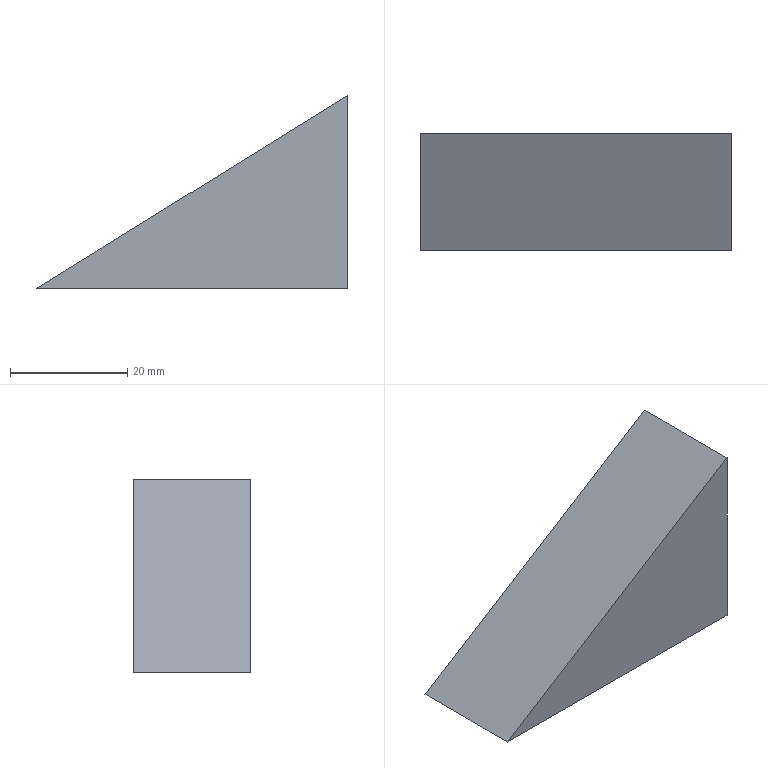Part | SolidWorks | features FlatPattern 1, SMBaseFlange 1, SheetMetal 1 | 1 solid | 5 faces | box 53 x 20 x 33 mm | volume 17490 mm3 | plane 5
STEP:
#1=CARTESIAN_POINT('',(0.,0.,0.));
#2=VERTEX_POINT('',#1);
#3=CARTESIAN_POINT('',(53.,0.,33.));
#4=VERTEX_POINT('',#3);
#5=CARTESIAN_POINT('',(53.,0.,33.));
#6=DIRECTION('',(0.8489,0.,0.5286));
#7=VECTOR('',#6,1000.);
#8=LINE('',#5,#7);
#9=EDGE_CURVE('',#2,#4,#8,.T.);
#10=ORIENTED_EDGE('',*,*,#9,.F.);
#11=CARTESIAN_POINT('',(0.,-20.,0.));
#12=VERTEX_POINT('',#11);
#13=CARTESIAN_POINT('',(0.,-20.,0.));
#14=DIRECTION('',(0.,1.,0.));
#15=VECTOR('',#14,1000.);
#16=LINE('',#13,#15);
#17=EDGE_CURVE('',#12,#2,#16,.T.);
#18=ORIENTED_EDGE('',*,*,#17,.F.);
#19=CARTESIAN_POINT('',(53.,-20.,33.));
#20=VERTEX_POINT('',#19);
#21=CARTESIAN_POINT('',(53.,-20.,33.));
#22=DIRECTION('',(0.8489,0.,0.5286));
#23=VECTOR('',#22,1000.);
#24=LINE('',#21,#23);
#25=EDGE_CURVE('',#12,#20,#24,.T.);
#26=ORIENTED_EDGE('',*,*,#25,.T.);
#27=CARTESIAN_POINT('',(53.,-20.,33.));
#28=DIRECTION('',(0.,1.,0.));
#29=VECTOR('',#28,1000.);
#30=LINE('',#27,#29);
#31=EDGE_CURVE('',#20,#4,#30,.T.);
#32=ORIENTED_EDGE('',*,*,#31,.T.);
#33=EDGE_LOOP('',(#10,#18,#26,#32));
#34=FACE_OUTER_BOUND('',#33,.T.);
#35=CARTESIAN_POINT('',(53.,-20.,33.));
#36=DIRECTION('',(-0.5286,0.,0.8489));
#37=DIRECTION('',(0.8489,0.,0.5286));
#38=AXIS2_PLACEMENT_3D('',#35,#36,#37);
#39=PLANE('',#38);
#40=ADVANCED_FACE('',(#34),#39,.T.);
#41=CARTESIAN_POINT('',(53.,0.,0.));
#42=VERTEX_POINT('',#41);
#43=CARTESIAN_POINT('',(0.,0.,0.));
#44=DIRECTION('',(-1.,0.,0.));
#45=VECTOR('',#44,1000.);
#46=LINE('',#43,#45);
#47=EDGE_CURVE('',#42,#2,#46,.T.);
#48=ORIENTED_EDGE('',*,*,#47,.F.);
#49=CARTESIAN_POINT('',(53.,-20.,0.));
#50=VERTEX_POINT('',#49);
#51=CARTESIAN_POINT('',(53.,-20.,0.));
#52=DIRECTION('',(0.,1.,0.));
#53=VECTOR('',#52,1000.);
#54=LINE('',#51,#53);
#55=EDGE_CURVE('',#50,#42,#54,.T.);
#56=ORIENTED_EDGE('',*,*,#55,.F.);
#57=CARTESIAN_POINT('',(0.,-20.,0.));
#58=DIRECTION('',(-1.,0.,0.));
#59=VECTOR('',#58,1000.);
#60=LINE('',#57,#59);
#61=EDGE_CURVE('',#50,#12,#60,.T.);
#62=ORIENTED_EDGE('',*,*,#61,.T.);
#63=ORIENTED_EDGE('',*,*,#17,.T.);
#64=EDGE_LOOP('',(#48,#56,#62,#63));
#65=FACE_OUTER_BOUND('',#64,.T.);
#66=CARTESIAN_POINT('',(0.,-20.,0.));
#67=DIRECTION('',(0.,0.,-1.));
#68=DIRECTION('',(-1.,0.,0.));
#69=AXIS2_PLACEMENT_3D('',#66,#67,#68);
#70=PLANE('',#69);
#71=ADVANCED_FACE('',(#65),#70,.T.);
#72=CARTESIAN_POINT('',(53.,0.,0.));
#73=DIRECTION('',(0.,0.,-1.));
#74=VECTOR('',#73,1000.);
#75=LINE('',#72,#74);
#76=EDGE_CURVE('',#4,#42,#75,.T.);
#77=ORIENTED_EDGE('',*,*,#76,.F.);
#78=ORIENTED_EDGE('',*,*,#31,.F.);
#79=CARTESIAN_POINT('',(53.,-20.,0.));
#80=DIRECTION('',(0.,0.,-1.));
#81=VECTOR('',#80,1000.);
#82=LINE('',#79,#81);
#83=EDGE_CURVE('',#20,#50,#82,.T.);
#84=ORIENTED_EDGE('',*,*,#83,.T.);
#85=ORIENTED_EDGE('',*,*,#55,.T.);
#86=EDGE_LOOP('',(#77,#78,#84,#85));
#87=FACE_OUTER_BOUND('',#86,.T.);
#88=CARTESIAN_POINT('',(53.,-20.,0.));
#89=DIRECTION('',(1.,0.,0.));
#90=DIRECTION('',(0.,0.,-1.));
#91=AXIS2_PLACEMENT_3D('',#88,#89,#90);
#92=PLANE('',#91);
#93=ADVANCED_FACE('',(#87),#92,.T.);
#94=ORIENTED_EDGE('',*,*,#25,.F.);
#95=ORIENTED_EDGE('',*,*,#61,.F.);
#96=ORIENTED_EDGE('',*,*,#83,.F.);
#97=EDGE_LOOP('',(#94,#95,#96));
#98=FACE_OUTER_BOUND('',#97,.T.);
#99=CARTESIAN_POINT('',(0.,-20.,0.));
#100=DIRECTION('',(0.,1.,0.));
#101=DIRECTION('',(0.,0.,1.));
#102=AXIS2_PLACEMENT_3D('',#99,#100,#101);
#103=PLANE('',#102);
#104=ADVANCED_FACE('',(#98),#103,.F.);
#105=ORIENTED_EDGE('',*,*,#9,.T.);
#106=ORIENTED_EDGE('',*,*,#76,.T.);
#107=ORIENTED_EDGE('',*,*,#47,.T.);
#108=EDGE_LOOP('',(#105,#106,#107));
#109=FACE_OUTER_BOUND('',#108,.T.);
#110=CARTESIAN_POINT('',(0.,0.,0.));
#111=DIRECTION('',(0.,1.,0.));
#112=DIRECTION('',(0.,0.,1.));
#113=AXIS2_PLACEMENT_3D('',#110,#111,#112);
#114=PLANE('',#113);
#115=ADVANCED_FACE('',(#109),#114,.T.);
#116=CLOSED_SHELL('',(#40,#71,#93,#104,#115));
#117=MANIFOLD_SOLID_BREP('',#116);
#118=CARTESIAN_POINT('',(0.,0.,0.));
#119=DIRECTION('',(0.,0.,1.));
#120=DIRECTION('',(1.,0.,0.));
#121=AXIS2_PLACEMENT_3D('',#118,#119,#120);
#122=(LENGTH_UNIT()NAMED_UNIT(*)SI_UNIT(.MILLI.,.METRE.));
#123=UNCERTAINTY_MEASURE_WITH_UNIT(LENGTH_MEASURE(0.00001),#122,'','');
#124=(NAMED_UNIT(*)PLANE_ANGLE_UNIT()SI_UNIT($,.RADIAN.));
#125=(NAMED_UNIT(*)SI_UNIT($,.STERADIAN.)SOLID_ANGLE_UNIT());
#126=(GEOMETRIC_REPRESENTATION_CONTEXT(3)GLOBAL_UNCERTAINTY_ASSIGNED_CONTEXT((#123))GLOBAL_UNIT_ASSIGNED_CONTEXT((#122,#124,#125))REPRESENTATION_CONTEXT('',''));
#127=ADVANCED_BREP_SHAPE_REPRESENTATION('',(#117,#121),#126);